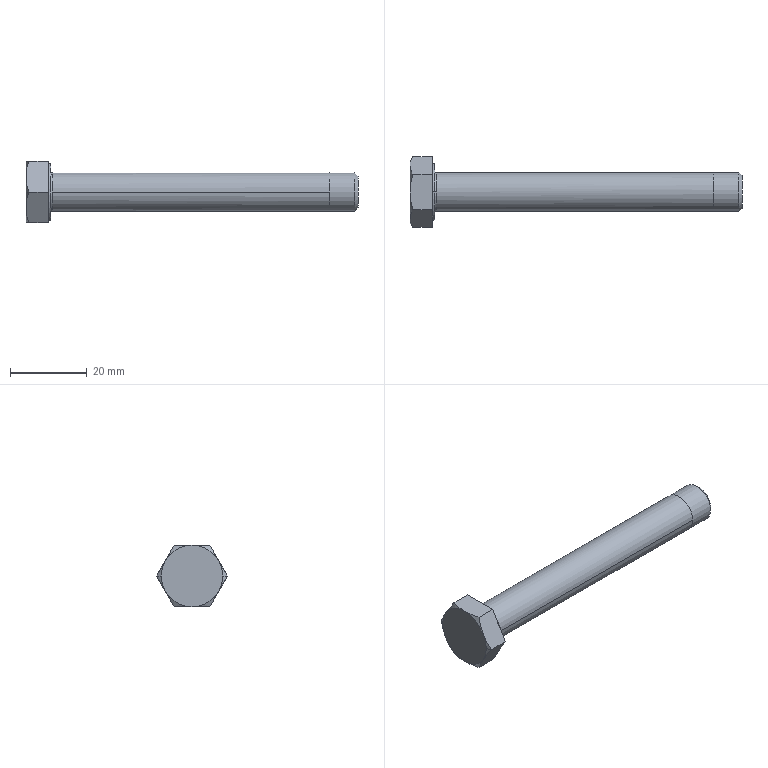Part | NX | features BREP 1, MOVE_FACE 1, REPLACE_FACE 1 | 1 solid | 27 faces | box 86.4 x 18.475 x 16 mm | volume 7660 mm3 | cone 10 | plane 10 | torus 4 | cylinder 3 | commonest cylinder face diameters 10 x3
STEP:
#1=CARTESIAN_POINT('',(-5.085,-9.238,0.));
#2=VERTEX_POINT('',#1);
#3=CARTESIAN_POINT('',(-5.8,-8.,0.));
#4=VERTEX_POINT('',#3);
#5=CARTESIAN_POINT('',(-5.442,-8.62,0.));
#6=DIRECTION('',(-0.5,0.866,0.));
#7=VECTOR('',#6,1000.);
#8=LINE('',#5,#7);
#9=EDGE_CURVE('',#2,#4,#8,.T.);
#10=ORIENTED_EDGE('',*,*,#9,.F.);
#11=CARTESIAN_POINT('',(-5.8,-6.928,4.));
#12=VERTEX_POINT('',#11);
#13=CARTESIAN_POINT('',(-5.084,-9.24,-0.004148));
#14=CARTESIAN_POINT('',(-5.8,-8.001,2.142));
#15=CARTESIAN_POINT('',(-5.8,-6.928,4.));
#16=CARTESIAN_POINT('',(-5.8,-5.855,5.858));
#17=CARTESIAN_POINT('',(-5.084,-4.616,8.004));
#18=(BOUNDED_CURVE()B_SPLINE_CURVE(2,(#13,#14,#15,#16,#17),.UNSPECIFIED.,.F.,.F.)B_SPLINE_CURVE_WITH_KNOTS((3,2,3),(0.,0.5,1.),.PIECEWISE_BEZIER_KNOTS.)CURVE()GEOMETRIC_REPRESENTATION_ITEM()RATIONAL_B_SPLINE_CURVE((1.,1.038,1.,1.038,1.))REPRESENTATION_ITEM(''));
#19=EDGE_CURVE('',#2,#12,#18,.T.);
#20=ORIENTED_EDGE('',*,*,#19,.T.);
#21=CARTESIAN_POINT('',(-5.8,0.,0.));
#22=DIRECTION('',(1.,0.,0.));
#23=DIRECTION('',(0.,1.,0.));
#24=AXIS2_PLACEMENT_3D('',#21,#22,#23);
#25=CIRCLE('',#24,8.);
#26=EDGE_CURVE('',#12,#4,#25,.T.);
#27=ORIENTED_EDGE('',*,*,#26,.T.);
#28=EDGE_LOOP('',(#10,#20,#27));
#29=FACE_BOUND('',#28,.T.);
#30=CARTESIAN_POINT('',(-5.442,0.,0.));
#31=DIRECTION('',(1.,0.,0.));
#32=DIRECTION('',(0.,-1.,0.));
#33=AXIS2_PLACEMENT_3D('',#30,#31,#32);
#34=CONICAL_SURFACE('',#33,8.62,1.047);
#35=ADVANCED_FACE('',(#29),#34,.T.);
#36=CARTESIAN_POINT('',(-5.8,8.,0.));
#37=VERTEX_POINT('',#36);
#38=CARTESIAN_POINT('',(-5.085,9.238,0.));
#39=VERTEX_POINT('',#38);
#40=CARTESIAN_POINT('',(-5.442,8.62,0.));
#41=DIRECTION('',(0.5,0.866,0.));
#42=VECTOR('',#41,1000.);
#43=LINE('',#40,#42);
#44=EDGE_CURVE('',#37,#39,#43,.T.);
#45=ORIENTED_EDGE('',*,*,#44,.F.);
#46=CARTESIAN_POINT('',(-5.8,6.928,4.));
#47=VERTEX_POINT('',#46);
#48=CARTESIAN_POINT('',(-5.8,0.,0.));
#49=DIRECTION('',(1.,0.,0.));
#50=DIRECTION('',(0.,1.,0.));
#51=AXIS2_PLACEMENT_3D('',#48,#49,#50);
#52=CIRCLE('',#51,8.);
#53=EDGE_CURVE('',#37,#47,#52,.T.);
#54=ORIENTED_EDGE('',*,*,#53,.T.);
#55=CARTESIAN_POINT('',(-5.084,4.616,8.004));
#56=CARTESIAN_POINT('',(-5.8,5.855,5.858));
#57=CARTESIAN_POINT('',(-5.8,6.928,4.));
#58=CARTESIAN_POINT('',(-5.8,8.001,2.142));
#59=CARTESIAN_POINT('',(-5.084,9.24,-0.004148));
#60=(BOUNDED_CURVE()B_SPLINE_CURVE(2,(#55,#56,#57,#58,#59),.UNSPECIFIED.,.F.,.F.)B_SPLINE_CURVE_WITH_KNOTS((3,2,3),(0.,0.5,1.),.PIECEWISE_BEZIER_KNOTS.)CURVE()GEOMETRIC_REPRESENTATION_ITEM()RATIONAL_B_SPLINE_CURVE((1.,1.038,1.,1.038,1.))REPRESENTATION_ITEM(''));
#61=EDGE_CURVE('',#47,#39,#60,.T.);
#62=ORIENTED_EDGE('',*,*,#61,.T.);
#63=EDGE_LOOP('',(#45,#54,#62));
#64=FACE_BOUND('',#63,.T.);
#65=CARTESIAN_POINT('',(-5.442,0.,0.));
#66=DIRECTION('',(1.,0.,0.));
#67=DIRECTION('',(0.,-1.,0.));
#68=AXIS2_PLACEMENT_3D('',#65,#66,#67);
#69=CONICAL_SURFACE('',#68,8.62,1.047);
#70=ADVANCED_FACE('',(#64),#69,.T.);
#71=CARTESIAN_POINT('',(79.788,5.,0.));
#72=VERTEX_POINT('',#71);
#73=CARTESIAN_POINT('',(80.6,4.188,0.));
#74=VERTEX_POINT('',#73);
#75=CARTESIAN_POINT('',(80.194,4.594,0.));
#76=DIRECTION('',(0.7071,-0.7071,0.));
#77=VECTOR('',#76,1000.);
#78=LINE('',#75,#77);
#79=EDGE_CURVE('',#72,#74,#78,.T.);
#80=ORIENTED_EDGE('',*,*,#79,.F.);
#81=CARTESIAN_POINT('',(79.788,-5.,0.));
#82=VERTEX_POINT('',#81);
#83=CARTESIAN_POINT('',(79.788,0.,0.));
#84=DIRECTION('',(1.,0.,0.));
#85=DIRECTION('',(0.,1.,0.));
#86=AXIS2_PLACEMENT_3D('',#83,#84,#85);
#87=CIRCLE('',#86,5.);
#88=EDGE_CURVE('',#72,#82,#87,.T.);
#89=ORIENTED_EDGE('',*,*,#88,.T.);
#90=CARTESIAN_POINT('',(80.6,-4.188,0.));
#91=VERTEX_POINT('',#90);
#92=CARTESIAN_POINT('',(80.194,-4.594,0.));
#93=DIRECTION('',(-0.7071,-0.7071,0.));
#94=VECTOR('',#93,1000.);
#95=LINE('',#92,#94);
#96=EDGE_CURVE('',#91,#82,#95,.T.);
#97=ORIENTED_EDGE('',*,*,#96,.F.);
#98=CARTESIAN_POINT('',(80.6,0.,0.));
#99=DIRECTION('',(1.,0.,0.));
#100=DIRECTION('',(0.,1.,0.));
#101=AXIS2_PLACEMENT_3D('',#98,#99,#100);
#102=CIRCLE('',#101,4.188);
#103=EDGE_CURVE('',#74,#91,#102,.T.);
#104=ORIENTED_EDGE('',*,*,#103,.F.);
#105=EDGE_LOOP('',(#80,#89,#97,#104));
#106=FACE_BOUND('',#105,.T.);
#107=CARTESIAN_POINT('',(80.194,0.,0.));
#108=DIRECTION('',(-1.,0.,0.));
#109=DIRECTION('',(0.,-1.,0.));
#110=AXIS2_PLACEMENT_3D('',#107,#108,#109);
#111=CONICAL_SURFACE('',#110,4.594,0.7854);
#112=ADVANCED_FACE('',(#106),#111,.T.);
#113=ORIENTED_EDGE('',*,*,#88,.F.);
#114=CARTESIAN_POINT('',(79.788,0.,0.));
#115=DIRECTION('',(1.,0.,0.));
#116=DIRECTION('',(0.,1.,0.));
#117=AXIS2_PLACEMENT_3D('',#114,#115,#116);
#118=CIRCLE('',#117,5.);
#119=EDGE_CURVE('',#82,#72,#118,.T.);
#120=ORIENTED_EDGE('',*,*,#119,.F.);
#121=EDGE_LOOP('',(#113,#120));
#122=FACE_BOUND('',#121,.T.);
#123=CARTESIAN_POINT('',(73.194,5.,0.));
#124=VERTEX_POINT('',#123);
#125=CARTESIAN_POINT('',(73.194,-5.,0.));
#126=VERTEX_POINT('',#125);
#127=CARTESIAN_POINT('',(73.194,0.,0.));
#128=DIRECTION('',(1.,0.,0.));
#129=DIRECTION('',(0.,1.,0.));
#130=AXIS2_PLACEMENT_3D('',#127,#128,#129);
#131=CIRCLE('',#130,5.);
#132=EDGE_CURVE('',#124,#126,#131,.T.);
#133=ORIENTED_EDGE('',*,*,#132,.T.);
#134=CARTESIAN_POINT('',(73.194,0.,0.));
#135=DIRECTION('',(1.,0.,0.));
#136=DIRECTION('',(0.,1.,0.));
#137=AXIS2_PLACEMENT_3D('',#134,#135,#136);
#138=CIRCLE('',#137,5.);
#139=EDGE_CURVE('',#126,#124,#138,.T.);
#140=ORIENTED_EDGE('',*,*,#139,.T.);
#141=EDGE_LOOP('',(#133,#140));
#142=FACE_BOUND('',#141,.T.);
#143=CARTESIAN_POINT('',(87.194,0.,0.));
#144=DIRECTION('',(1.,0.,0.));
#145=DIRECTION('',(0.,-1.,0.));
#146=AXIS2_PLACEMENT_3D('',#143,#144,#145);
#147=CYLINDRICAL_SURFACE('',#146,5.);
#148=ADVANCED_FACE('',(#122,#142),#147,.T.);
#149=CARTESIAN_POINT('',(1.,5.,0.));
#150=VERTEX_POINT('',#149);
#151=CARTESIAN_POINT('',(37.097,5.,0.));
#152=DIRECTION('',(1.,0.,0.));
#153=VECTOR('',#152,1000.);
#154=LINE('',#151,#153);
#155=EDGE_CURVE('',#150,#124,#154,.T.);
#156=ORIENTED_EDGE('',*,*,#155,.F.);
#157=CARTESIAN_POINT('',(1.,0.,5.));
#158=VERTEX_POINT('',#157);
#159=CARTESIAN_POINT('',(1.,0.,0.));
#160=DIRECTION('',(1.,0.,0.));
#161=DIRECTION('',(0.,1.,0.));
#162=AXIS2_PLACEMENT_3D('',#159,#160,#161);
#163=CIRCLE('',#162,5.);
#164=EDGE_CURVE('',#150,#158,#163,.T.);
#165=ORIENTED_EDGE('',*,*,#164,.T.);
#166=CARTESIAN_POINT('',(1.,-5.,0.));
#167=VERTEX_POINT('',#166);
#168=CARTESIAN_POINT('',(1.,0.,0.));
#169=DIRECTION('',(1.,0.,0.));
#170=DIRECTION('',(0.,1.,0.));
#171=AXIS2_PLACEMENT_3D('',#168,#169,#170);
#172=CIRCLE('',#171,5.);
#173=EDGE_CURVE('',#158,#167,#172,.T.);
#174=ORIENTED_EDGE('',*,*,#173,.T.);
#175=CARTESIAN_POINT('',(37.097,-5.,0.));
#176=DIRECTION('',(-1.,0.,0.));
#177=VECTOR('',#176,1000.);
#178=LINE('',#175,#177);
#179=EDGE_CURVE('',#126,#167,#178,.T.);
#180=ORIENTED_EDGE('',*,*,#179,.F.);
#181=ORIENTED_EDGE('',*,*,#132,.F.);
#182=EDGE_LOOP('',(#156,#165,#174,#180,#181));
#183=FACE_BOUND('',#182,.T.);
#184=CARTESIAN_POINT('',(37.097,0.,0.));
#185=DIRECTION('',(1.,0.,0.));
#186=DIRECTION('',(0.,-1.,0.));
#187=AXIS2_PLACEMENT_3D('',#184,#185,#186);
#188=CYLINDRICAL_SURFACE('',#187,5.);
#189=ADVANCED_FACE('',(#183),#188,.T.);
#190=CARTESIAN_POINT('',(0.6,0.,5.4));
#191=VERTEX_POINT('',#190);
#192=CARTESIAN_POINT('',(1.,0.,5.4));
#193=DIRECTION('',(0.,-1.,0.));
#194=DIRECTION('',(0.,0.,1.));
#195=AXIS2_PLACEMENT_3D('',#192,#193,#194);
#196=CIRCLE('',#195,0.4);
#197=EDGE_CURVE('',#191,#158,#196,.T.);
#198=ORIENTED_EDGE('',*,*,#197,.F.);
#199=CARTESIAN_POINT('',(0.6,0.,-5.4));
#200=VERTEX_POINT('',#199);
#201=CARTESIAN_POINT('',(0.6,0.,0.));
#202=DIRECTION('',(1.,0.,0.));
#203=DIRECTION('',(0.,1.,0.));
#204=AXIS2_PLACEMENT_3D('',#201,#202,#203);
#205=CIRCLE('',#204,5.4);
#206=EDGE_CURVE('',#191,#200,#205,.T.);
#207=ORIENTED_EDGE('',*,*,#206,.T.);
#208=CARTESIAN_POINT('',(1.,0.,-5.));
#209=VERTEX_POINT('',#208);
#210=CARTESIAN_POINT('',(1.,0.,-5.4));
#211=DIRECTION('',(0.,-1.,0.));
#212=DIRECTION('',(0.,0.,-1.));
#213=AXIS2_PLACEMENT_3D('',#210,#211,#212);
#214=CIRCLE('',#213,0.4);
#215=EDGE_CURVE('',#209,#200,#214,.T.);
#216=ORIENTED_EDGE('',*,*,#215,.F.);
#217=CARTESIAN_POINT('',(1.,0.,0.));
#218=DIRECTION('',(1.,0.,0.));
#219=DIRECTION('',(0.,1.,0.));
#220=AXIS2_PLACEMENT_3D('',#217,#218,#219);
#221=CIRCLE('',#220,5.);
#222=EDGE_CURVE('',#167,#209,#221,.T.);
#223=ORIENTED_EDGE('',*,*,#222,.F.);
#224=ORIENTED_EDGE('',*,*,#173,.F.);
#225=EDGE_LOOP('',(#198,#207,#216,#223,#224));
#226=FACE_BOUND('',#225,.T.);
#227=CARTESIAN_POINT('',(1.,0.,0.));
#228=DIRECTION('',(1.,0.,0.));
#229=DIRECTION('',(0.,0.,1.));
#230=AXIS2_PLACEMENT_3D('',#227,#228,#229);
#231=TOROIDAL_SURFACE('',#230,5.4,0.4);
#232=ADVANCED_FACE('',(#226),#231,.F.);
#233=CARTESIAN_POINT('',(0.,0.,7.915));
#234=VERTEX_POINT('',#233);
#235=CARTESIAN_POINT('',(0.6,0.,7.315));
#236=VERTEX_POINT('',#235);
#237=CARTESIAN_POINT('',(0.6,0.,7.915));
#238=DIRECTION('',(0.,-1.,0.));
#239=DIRECTION('',(0.,0.,1.));
#240=AXIS2_PLACEMENT_3D('',#237,#238,#239);
#241=CIRCLE('',#240,0.6);
#242=EDGE_CURVE('',#234,#236,#241,.T.);
#243=ORIENTED_EDGE('',*,*,#242,.F.);
#244=CARTESIAN_POINT('',(0.,0.,-7.915));
#245=VERTEX_POINT('',#244);
#246=CARTESIAN_POINT('',(0.,0.,0.));
#247=DIRECTION('',(-1.,0.,0.));
#248=DIRECTION('',(0.,1.,0.));
#249=AXIS2_PLACEMENT_3D('',#246,#247,#248);
#250=CIRCLE('',#249,7.915);
#251=EDGE_CURVE('',#245,#234,#250,.T.);
#252=ORIENTED_EDGE('',*,*,#251,.F.);
#253=CARTESIAN_POINT('',(0.6,0.,-7.315));
#254=VERTEX_POINT('',#253);
#255=CARTESIAN_POINT('',(0.6,0.,-7.915));
#256=DIRECTION('',(0.,-1.,0.));
#257=DIRECTION('',(0.,0.,-1.));
#258=AXIS2_PLACEMENT_3D('',#255,#256,#257);
#259=CIRCLE('',#258,0.6);
#260=EDGE_CURVE('',#254,#245,#259,.T.);
#261=ORIENTED_EDGE('',*,*,#260,.F.);
#262=CARTESIAN_POINT('',(0.6,0.,0.));
#263=DIRECTION('',(1.,0.,0.));
#264=DIRECTION('',(0.,1.,0.));
#265=AXIS2_PLACEMENT_3D('',#262,#263,#264);
#266=CIRCLE('',#265,7.315);
#267=EDGE_CURVE('',#236,#254,#266,.T.);
#268=ORIENTED_EDGE('',*,*,#267,.F.);
#269=EDGE_LOOP('',(#243,#252,#261,#268));
#270=FACE_BOUND('',#269,.T.);
#271=CARTESIAN_POINT('',(0.6,0.,0.));
#272=DIRECTION('',(1.,0.,0.));
#273=DIRECTION('',(0.,0.,1.));
#274=AXIS2_PLACEMENT_3D('',#271,#272,#273);
#275=TOROIDAL_SURFACE('',#274,7.915,0.6);
#276=ADVANCED_FACE('',(#270),#275,.F.);
#277=ORIENTED_EDGE('',*,*,#242,.T.);
#278=CARTESIAN_POINT('',(0.6,7.315,0.));
#279=VERTEX_POINT('',#278);
#280=CARTESIAN_POINT('',(0.6,0.,0.));
#281=DIRECTION('',(1.,0.,0.));
#282=DIRECTION('',(0.,1.,0.));
#283=AXIS2_PLACEMENT_3D('',#280,#281,#282);
#284=CIRCLE('',#283,7.315);
#285=EDGE_CURVE('',#279,#236,#284,.T.);
#286=ORIENTED_EDGE('',*,*,#285,.F.);
#287=CARTESIAN_POINT('',(0.6,0.,0.));
#288=DIRECTION('',(1.,0.,0.));
#289=DIRECTION('',(0.,1.,0.));
#290=AXIS2_PLACEMENT_3D('',#287,#288,#289);
#291=CIRCLE('',#290,7.315);
#292=EDGE_CURVE('',#254,#279,#291,.T.);
#293=ORIENTED_EDGE('',*,*,#292,.F.);
#294=ORIENTED_EDGE('',*,*,#260,.T.);
#295=CARTESIAN_POINT('',(0.,7.915,0.));
#296=VERTEX_POINT('',#295);
#297=CARTESIAN_POINT('',(0.,0.,0.));
#298=DIRECTION('',(-1.,0.,0.));
#299=DIRECTION('',(0.,1.,0.));
#300=AXIS2_PLACEMENT_3D('',#297,#298,#299);
#301=CIRCLE('',#300,7.915);
#302=EDGE_CURVE('',#296,#245,#301,.T.);
#303=ORIENTED_EDGE('',*,*,#302,.F.);
#304=CARTESIAN_POINT('',(0.,0.,0.));
#305=DIRECTION('',(-1.,0.,0.));
#306=DIRECTION('',(0.,1.,0.));
#307=AXIS2_PLACEMENT_3D('',#304,#305,#306);
#308=CIRCLE('',#307,7.915);
#309=EDGE_CURVE('',#234,#296,#308,.T.);
#310=ORIENTED_EDGE('',*,*,#309,.F.);
#311=EDGE_LOOP('',(#277,#286,#293,#294,#303,#310));
#312=FACE_BOUND('',#311,.T.);
#313=CARTESIAN_POINT('',(0.6,0.,0.));
#314=DIRECTION('',(1.,0.,0.));
#315=DIRECTION('',(0.,0.,1.));
#316=AXIS2_PLACEMENT_3D('',#313,#314,#315);
#317=TOROIDAL_SURFACE('',#316,7.915,0.6);
#318=ADVANCED_FACE('',(#312),#317,.F.);
#319=CARTESIAN_POINT('',(0.6,5.4,0.));
#320=VERTEX_POINT('',#319);
#321=CARTESIAN_POINT('',(0.6,0.,0.));
#322=DIRECTION('',(1.,0.,0.));
#323=DIRECTION('',(0.,1.,0.));
#324=AXIS2_PLACEMENT_3D('',#321,#322,#323);
#325=CIRCLE('',#324,5.4);
#326=EDGE_CURVE('',#320,#191,#325,.T.);
#327=ORIENTED_EDGE('',*,*,#326,.F.);
#328=CARTESIAN_POINT('',(0.6,0.,0.));
#329=DIRECTION('',(1.,0.,0.));
#330=DIRECTION('',(0.,1.,0.));
#331=AXIS2_PLACEMENT_3D('',#328,#329,#330);
#332=CIRCLE('',#331,5.4);
#333=EDGE_CURVE('',#200,#320,#332,.T.);
#334=ORIENTED_EDGE('',*,*,#333,.F.);
#335=ORIENTED_EDGE('',*,*,#206,.F.);
#336=EDGE_LOOP('',(#327,#334,#335));
#337=FACE_BOUND('',#336,.T.);
#338=ORIENTED_EDGE('',*,*,#285,.T.);
#339=ORIENTED_EDGE('',*,*,#267,.T.);
#340=ORIENTED_EDGE('',*,*,#292,.T.);
#341=EDGE_LOOP('',(#338,#339,#340));
#342=FACE_BOUND('',#341,.T.);
#343=CARTESIAN_POINT('',(0.6,6.357,0.));
#344=DIRECTION('',(1.,0.,0.));
#345=DIRECTION('',(0.,-1.,0.));
#346=AXIS2_PLACEMENT_3D('',#343,#344,#345);
#347=PLANE('',#346);
#348=ADVANCED_FACE('',(#337,#342),#347,.T.);
#349=ORIENTED_EDGE('',*,*,#197,.T.);
#350=ORIENTED_EDGE('',*,*,#164,.F.);
#351=CARTESIAN_POINT('',(1.,0.,0.));
#352=DIRECTION('',(1.,0.,0.));
#353=DIRECTION('',(0.,1.,0.));
#354=AXIS2_PLACEMENT_3D('',#351,#352,#353);
#355=CIRCLE('',#354,5.);
#356=EDGE_CURVE('',#209,#150,#355,.T.);
#357=ORIENTED_EDGE('',*,*,#356,.F.);
#358=ORIENTED_EDGE('',*,*,#215,.T.);
#359=ORIENTED_EDGE('',*,*,#333,.T.);
#360=ORIENTED_EDGE('',*,*,#326,.T.);
#361=EDGE_LOOP('',(#349,#350,#357,#358,#359,#360));
#362=FACE_BOUND('',#361,.T.);
#363=CARTESIAN_POINT('',(1.,0.,0.));
#364=DIRECTION('',(1.,0.,0.));
#365=DIRECTION('',(0.,0.,1.));
#366=AXIS2_PLACEMENT_3D('',#363,#364,#365);
#367=TOROIDAL_SURFACE('',#366,5.4,0.4);
#368=ADVANCED_FACE('',(#362),#367,.F.);
#369=ORIENTED_EDGE('',*,*,#155,.T.);
#370=ORIENTED_EDGE('',*,*,#139,.F.);
#371=ORIENTED_EDGE('',*,*,#179,.T.);
#372=ORIENTED_EDGE('',*,*,#222,.T.);
#373=ORIENTED_EDGE('',*,*,#356,.T.);
#374=EDGE_LOOP('',(#369,#370,#371,#372,#373));
#375=FACE_BOUND('',#374,.T.);
#376=CARTESIAN_POINT('',(37.097,0.,0.));
#377=DIRECTION('',(1.,0.,0.));
#378=DIRECTION('',(0.,-1.,0.));
#379=AXIS2_PLACEMENT_3D('',#376,#377,#378);
#380=CYLINDRICAL_SURFACE('',#379,5.);
#381=ADVANCED_FACE('',(#375),#380,.T.);
#382=ORIENTED_EDGE('',*,*,#79,.T.);
#383=CARTESIAN_POINT('',(80.6,0.,0.));
#384=DIRECTION('',(1.,0.,0.));
#385=DIRECTION('',(0.,1.,0.));
#386=AXIS2_PLACEMENT_3D('',#383,#384,#385);
#387=CIRCLE('',#386,4.188);
#388=EDGE_CURVE('',#91,#74,#387,.T.);
#389=ORIENTED_EDGE('',*,*,#388,.F.);
#390=ORIENTED_EDGE('',*,*,#96,.T.);
#391=ORIENTED_EDGE('',*,*,#119,.T.);
#392=EDGE_LOOP('',(#382,#389,#390,#391));
#393=FACE_BOUND('',#392,.T.);
#394=CARTESIAN_POINT('',(80.194,0.,0.));
#395=DIRECTION('',(-1.,0.,0.));
#396=DIRECTION('',(0.,-1.,0.));
#397=AXIS2_PLACEMENT_3D('',#394,#395,#396);
#398=CONICAL_SURFACE('',#397,4.594,0.7854);
#399=ADVANCED_FACE('',(#393),#398,.T.);
#400=ORIENTED_EDGE('',*,*,#103,.T.);
#401=ORIENTED_EDGE('',*,*,#388,.T.);
#402=EDGE_LOOP('',(#400,#401));
#403=FACE_BOUND('',#402,.T.);
#404=CARTESIAN_POINT('',(80.6,2.094,0.));
#405=DIRECTION('',(1.,0.,0.));
#406=DIRECTION('',(0.,-1.,0.));
#407=AXIS2_PLACEMENT_3D('',#404,#405,#406);
#408=PLANE('',#407);
#409=ADVANCED_FACE('',(#403),#408,.T.);
#410=CARTESIAN_POINT('',(-5.085,-4.619,8.));
#411=VERTEX_POINT('',#410);
#412=CARTESIAN_POINT('',(-5.8,0.,8.));
#413=VERTEX_POINT('',#412);
#414=CARTESIAN_POINT('',(-5.084,-4.624,8.));
#415=CARTESIAN_POINT('',(-5.8,-2.146,8.));
#416=CARTESIAN_POINT('',(-5.8,0.,8.));
#417=CARTESIAN_POINT('',(-5.8,2.146,8.));
#418=CARTESIAN_POINT('',(-5.084,4.624,8.));
#419=(BOUNDED_CURVE()B_SPLINE_CURVE(2,(#414,#415,#416,#417,#418),.UNSPECIFIED.,.F.,.F.)B_SPLINE_CURVE_WITH_KNOTS((3,2,3),(0.,0.5,1.),.PIECEWISE_BEZIER_KNOTS.)CURVE()GEOMETRIC_REPRESENTATION_ITEM()RATIONAL_B_SPLINE_CURVE((1.,1.038,1.,1.038,1.))REPRESENTATION_ITEM(''));
#420=EDGE_CURVE('',#411,#413,#419,.T.);
#421=ORIENTED_EDGE('',*,*,#420,.T.);
#422=CARTESIAN_POINT('',(-5.8,0.,0.));
#423=DIRECTION('',(1.,0.,0.));
#424=DIRECTION('',(0.,1.,0.));
#425=AXIS2_PLACEMENT_3D('',#422,#423,#424);
#426=CIRCLE('',#425,8.);
#427=EDGE_CURVE('',#413,#12,#426,.T.);
#428=ORIENTED_EDGE('',*,*,#427,.T.);
#429=CARTESIAN_POINT('',(-5.084,-9.24,-0.004148));
#430=CARTESIAN_POINT('',(-5.8,-8.001,2.142));
#431=CARTESIAN_POINT('',(-5.8,-6.928,4.));
#432=CARTESIAN_POINT('',(-5.8,-5.855,5.858));
#433=CARTESIAN_POINT('',(-5.084,-4.616,8.004));
#434=(BOUNDED_CURVE()B_SPLINE_CURVE(2,(#429,#430,#431,#432,#433),.UNSPECIFIED.,.F.,.F.)B_SPLINE_CURVE_WITH_KNOTS((3,2,3),(0.,0.5,1.),.PIECEWISE_BEZIER_KNOTS.)CURVE()GEOMETRIC_REPRESENTATION_ITEM()RATIONAL_B_SPLINE_CURVE((1.,1.038,1.,1.038,1.))REPRESENTATION_ITEM(''));
#435=EDGE_CURVE('',#12,#411,#434,.T.);
#436=ORIENTED_EDGE('',*,*,#435,.T.);
#437=EDGE_LOOP('',(#421,#428,#436));
#438=FACE_BOUND('',#437,.T.);
#439=CARTESIAN_POINT('',(-5.442,0.,0.));
#440=DIRECTION('',(1.,0.,0.));
#441=DIRECTION('',(0.,-1.,0.));
#442=AXIS2_PLACEMENT_3D('',#439,#440,#441);
#443=CONICAL_SURFACE('',#442,8.62,1.047);
#444=ADVANCED_FACE('',(#438),#443,.T.);
#445=CARTESIAN_POINT('',(-5.085,4.619,8.));
#446=VERTEX_POINT('',#445);
#447=CARTESIAN_POINT('',(-5.084,4.616,8.004));
#448=CARTESIAN_POINT('',(-5.8,5.855,5.858));
#449=CARTESIAN_POINT('',(-5.8,6.928,4.));
#450=CARTESIAN_POINT('',(-5.8,8.001,2.142));
#451=CARTESIAN_POINT('',(-5.084,9.24,-0.004148));
#452=(BOUNDED_CURVE()B_SPLINE_CURVE(2,(#447,#448,#449,#450,#451),.UNSPECIFIED.,.F.,.F.)B_SPLINE_CURVE_WITH_KNOTS((3,2,3),(0.,0.5,1.),.PIECEWISE_BEZIER_KNOTS.)CURVE()GEOMETRIC_REPRESENTATION_ITEM()RATIONAL_B_SPLINE_CURVE((1.,1.038,1.,1.038,1.))REPRESENTATION_ITEM(''));
#453=EDGE_CURVE('',#446,#47,#452,.T.);
#454=ORIENTED_EDGE('',*,*,#453,.T.);
#455=CARTESIAN_POINT('',(-5.8,0.,0.));
#456=DIRECTION('',(1.,0.,0.));
#457=DIRECTION('',(0.,1.,0.));
#458=AXIS2_PLACEMENT_3D('',#455,#456,#457);
#459=CIRCLE('',#458,8.);
#460=EDGE_CURVE('',#47,#413,#459,.T.);
#461=ORIENTED_EDGE('',*,*,#460,.T.);
#462=CARTESIAN_POINT('',(-5.084,-4.624,8.));
#463=CARTESIAN_POINT('',(-5.8,-2.146,8.));
#464=CARTESIAN_POINT('',(-5.8,0.,8.));
#465=CARTESIAN_POINT('',(-5.8,2.146,8.));
#466=CARTESIAN_POINT('',(-5.084,4.624,8.));
#467=(BOUNDED_CURVE()B_SPLINE_CURVE(2,(#462,#463,#464,#465,#466),.UNSPECIFIED.,.F.,.F.)B_SPLINE_CURVE_WITH_KNOTS((3,2,3),(0.,0.5,1.),.PIECEWISE_BEZIER_KNOTS.)CURVE()GEOMETRIC_REPRESENTATION_ITEM()RATIONAL_B_SPLINE_CURVE((1.,1.038,1.,1.038,1.))REPRESENTATION_ITEM(''));
#468=EDGE_CURVE('',#413,#446,#467,.T.);
#469=ORIENTED_EDGE('',*,*,#468,.T.);
#470=EDGE_LOOP('',(#454,#461,#469));
#471=FACE_BOUND('',#470,.T.);
#472=CARTESIAN_POINT('',(-5.442,0.,0.));
#473=DIRECTION('',(1.,0.,0.));
#474=DIRECTION('',(0.,-1.,0.));
#475=AXIS2_PLACEMENT_3D('',#472,#473,#474);
#476=CONICAL_SURFACE('',#475,8.62,1.047);
#477=ADVANCED_FACE('',(#471),#476,.T.);
#478=ORIENTED_EDGE('',*,*,#44,.T.);
#479=CARTESIAN_POINT('',(-5.8,6.928,-4.));
#480=VERTEX_POINT('',#479);
#481=CARTESIAN_POINT('',(-5.084,9.24,0.004148));
#482=CARTESIAN_POINT('',(-5.8,8.001,-2.142));
#483=CARTESIAN_POINT('',(-5.8,6.928,-4.));
#484=CARTESIAN_POINT('',(-5.8,5.855,-5.858));
#485=CARTESIAN_POINT('',(-5.084,4.616,-8.004));
#486=(BOUNDED_CURVE()B_SPLINE_CURVE(2,(#481,#482,#483,#484,#485),.UNSPECIFIED.,.F.,.F.)B_SPLINE_CURVE_WITH_KNOTS((3,2,3),(0.,0.5,1.),.PIECEWISE_BEZIER_KNOTS.)CURVE()GEOMETRIC_REPRESENTATION_ITEM()RATIONAL_B_SPLINE_CURVE((1.,1.038,1.,1.038,1.))REPRESENTATION_ITEM(''));
#487=EDGE_CURVE('',#39,#480,#486,.T.);
#488=ORIENTED_EDGE('',*,*,#487,.T.);
#489=CARTESIAN_POINT('',(-5.8,0.,0.));
#490=DIRECTION('',(1.,0.,0.));
#491=DIRECTION('',(0.,1.,0.));
#492=AXIS2_PLACEMENT_3D('',#489,#490,#491);
#493=CIRCLE('',#492,8.);
#494=EDGE_CURVE('',#480,#37,#493,.T.);
#495=ORIENTED_EDGE('',*,*,#494,.T.);
#496=EDGE_LOOP('',(#478,#488,#495));
#497=FACE_BOUND('',#496,.T.);
#498=CARTESIAN_POINT('',(-5.442,0.,0.));
#499=DIRECTION('',(1.,0.,0.));
#500=DIRECTION('',(0.,-1.,0.));
#501=AXIS2_PLACEMENT_3D('',#498,#499,#500);
#502=CONICAL_SURFACE('',#501,8.62,1.047);
#503=ADVANCED_FACE('',(#497),#502,.T.);
#504=CARTESIAN_POINT('',(-5.085,4.619,-8.));
#505=VERTEX_POINT('',#504);
#506=CARTESIAN_POINT('',(-5.084,9.24,0.004148));
#507=CARTESIAN_POINT('',(-5.8,8.001,-2.142));
#508=CARTESIAN_POINT('',(-5.8,6.928,-4.));
#509=CARTESIAN_POINT('',(-5.8,5.855,-5.858));
#510=CARTESIAN_POINT('',(-5.084,4.616,-8.004));
#511=(BOUNDED_CURVE()B_SPLINE_CURVE(2,(#506,#507,#508,#509,#510),.UNSPECIFIED.,.F.,.F.)B_SPLINE_CURVE_WITH_KNOTS((3,2,3),(0.,0.5,1.),.PIECEWISE_BEZIER_KNOTS.)CURVE()GEOMETRIC_REPRESENTATION_ITEM()RATIONAL_B_SPLINE_CURVE((1.,1.038,1.,1.038,1.))REPRESENTATION_ITEM(''));
#512=EDGE_CURVE('',#480,#505,#511,.T.);
#513=ORIENTED_EDGE('',*,*,#512,.T.);
#514=CARTESIAN_POINT('',(-5.8,0.,-8.));
#515=VERTEX_POINT('',#514);
#516=CARTESIAN_POINT('',(-5.084,4.624,-8.));
#517=CARTESIAN_POINT('',(-5.8,2.146,-8.));
#518=CARTESIAN_POINT('',(-5.8,0.,-8.));
#519=CARTESIAN_POINT('',(-5.8,-2.146,-8.));
#520=CARTESIAN_POINT('',(-5.084,-4.624,-8.));
#521=(BOUNDED_CURVE()B_SPLINE_CURVE(2,(#516,#517,#518,#519,#520),.UNSPECIFIED.,.F.,.F.)B_SPLINE_CURVE_WITH_KNOTS((3,2,3),(0.,0.5,1.),.PIECEWISE_BEZIER_KNOTS.)CURVE()GEOMETRIC_REPRESENTATION_ITEM()RATIONAL_B_SPLINE_CURVE((1.,1.038,1.,1.038,1.))REPRESENTATION_ITEM(''));
#522=EDGE_CURVE('',#505,#515,#521,.T.);
#523=ORIENTED_EDGE('',*,*,#522,.T.);
#524=CARTESIAN_POINT('',(-5.8,0.,0.));
#525=DIRECTION('',(1.,0.,0.));
#526=DIRECTION('',(0.,1.,0.));
#527=AXIS2_PLACEMENT_3D('',#524,#525,#526);
#528=CIRCLE('',#527,8.);
#529=EDGE_CURVE('',#515,#480,#528,.T.);
#530=ORIENTED_EDGE('',*,*,#529,.T.);
#531=EDGE_LOOP('',(#513,#523,#530));
#532=FACE_BOUND('',#531,.T.);
#533=CARTESIAN_POINT('',(-5.442,0.,0.));
#534=DIRECTION('',(1.,0.,0.));
#535=DIRECTION('',(0.,-1.,0.));
#536=AXIS2_PLACEMENT_3D('',#533,#534,#535);
#537=CONICAL_SURFACE('',#536,8.62,1.047);
#538=ADVANCED_FACE('',(#532),#537,.T.);
#539=CARTESIAN_POINT('',(-5.085,-4.619,-8.));
#540=VERTEX_POINT('',#539);
#541=CARTESIAN_POINT('',(-5.084,4.624,-8.));
#542=CARTESIAN_POINT('',(-5.8,2.146,-8.));
#543=CARTESIAN_POINT('',(-5.8,0.,-8.));
#544=CARTESIAN_POINT('',(-5.8,-2.146,-8.));
#545=CARTESIAN_POINT('',(-5.084,-4.624,-8.));
#546=(BOUNDED_CURVE()B_SPLINE_CURVE(2,(#541,#542,#543,#544,#545),.UNSPECIFIED.,.F.,.F.)B_SPLINE_CURVE_WITH_KNOTS((3,2,3),(0.,0.5,1.),.PIECEWISE_BEZIER_KNOTS.)CURVE()GEOMETRIC_REPRESENTATION_ITEM()RATIONAL_B_SPLINE_CURVE((1.,1.038,1.,1.038,1.))REPRESENTATION_ITEM(''));
#547=EDGE_CURVE('',#515,#540,#546,.T.);
#548=ORIENTED_EDGE('',*,*,#547,.T.);
#549=CARTESIAN_POINT('',(-5.8,-6.928,-4.));
#550=VERTEX_POINT('',#549);
#551=CARTESIAN_POINT('',(-5.084,-4.616,-8.004));
#552=CARTESIAN_POINT('',(-5.8,-5.855,-5.858));
#553=CARTESIAN_POINT('',(-5.8,-6.928,-4.));
#554=CARTESIAN_POINT('',(-5.8,-8.001,-2.142));
#555=CARTESIAN_POINT('',(-5.084,-9.24,0.004148));
#556=(BOUNDED_CURVE()B_SPLINE_CURVE(2,(#551,#552,#553,#554,#555),.UNSPECIFIED.,.F.,.F.)B_SPLINE_CURVE_WITH_KNOTS((3,2,3),(0.,0.5,1.),.PIECEWISE_BEZIER_KNOTS.)CURVE()GEOMETRIC_REPRESENTATION_ITEM()RATIONAL_B_SPLINE_CURVE((1.,1.038,1.,1.038,1.))REPRESENTATION_ITEM(''));
#557=EDGE_CURVE('',#540,#550,#556,.T.);
#558=ORIENTED_EDGE('',*,*,#557,.T.);
#559=CARTESIAN_POINT('',(-5.8,0.,0.));
#560=DIRECTION('',(1.,0.,0.));
#561=DIRECTION('',(0.,1.,0.));
#562=AXIS2_PLACEMENT_3D('',#559,#560,#561);
#563=CIRCLE('',#562,8.);
#564=EDGE_CURVE('',#550,#515,#563,.T.);
#565=ORIENTED_EDGE('',*,*,#564,.T.);
#566=EDGE_LOOP('',(#548,#558,#565));
#567=FACE_BOUND('',#566,.T.);
#568=CARTESIAN_POINT('',(-5.442,0.,0.));
#569=DIRECTION('',(1.,0.,0.));
#570=DIRECTION('',(0.,-1.,0.));
#571=AXIS2_PLACEMENT_3D('',#568,#569,#570);
#572=CONICAL_SURFACE('',#571,8.62,1.047);
#573=ADVANCED_FACE('',(#567),#572,.T.);
#574=ORIENTED_EDGE('',*,*,#9,.T.);
#575=CARTESIAN_POINT('',(-5.8,0.,0.));
#576=DIRECTION('',(1.,0.,0.));
#577=DIRECTION('',(0.,1.,0.));
#578=AXIS2_PLACEMENT_3D('',#575,#576,#577);
#579=CIRCLE('',#578,8.);
#580=EDGE_CURVE('',#4,#550,#579,.T.);
#581=ORIENTED_EDGE('',*,*,#580,.T.);
#582=CARTESIAN_POINT('',(-5.084,-4.616,-8.004));
#583=CARTESIAN_POINT('',(-5.8,-5.855,-5.858));
#584=CARTESIAN_POINT('',(-5.8,-6.928,-4.));
#585=CARTESIAN_POINT('',(-5.8,-8.001,-2.142));
#586=CARTESIAN_POINT('',(-5.084,-9.24,0.004148));
#587=(BOUNDED_CURVE()B_SPLINE_CURVE(2,(#582,#583,#584,#585,#586),.UNSPECIFIED.,.F.,.F.)B_SPLINE_CURVE_WITH_KNOTS((3,2,3),(0.,0.5,1.),.PIECEWISE_BEZIER_KNOTS.)CURVE()GEOMETRIC_REPRESENTATION_ITEM()RATIONAL_B_SPLINE_CURVE((1.,1.038,1.,1.038,1.))REPRESENTATION_ITEM(''));
#588=EDGE_CURVE('',#550,#2,#587,.T.);
#589=ORIENTED_EDGE('',*,*,#588,.T.);
#590=EDGE_LOOP('',(#574,#581,#589));
#591=FACE_BOUND('',#590,.T.);
#592=CARTESIAN_POINT('',(-5.442,0.,0.));
#593=DIRECTION('',(1.,0.,0.));
#594=DIRECTION('',(0.,-1.,0.));
#595=AXIS2_PLACEMENT_3D('',#592,#593,#594);
#596=CONICAL_SURFACE('',#595,8.62,1.047);
#597=ADVANCED_FACE('',(#591),#596,.T.);
#598=ORIENTED_EDGE('',*,*,#494,.F.);
#599=ORIENTED_EDGE('',*,*,#529,.F.);
#600=ORIENTED_EDGE('',*,*,#564,.F.);
#601=ORIENTED_EDGE('',*,*,#580,.F.);
#602=ORIENTED_EDGE('',*,*,#26,.F.);
#603=ORIENTED_EDGE('',*,*,#427,.F.);
#604=ORIENTED_EDGE('',*,*,#460,.F.);
#605=ORIENTED_EDGE('',*,*,#53,.F.);
#606=EDGE_LOOP('',(#598,#599,#600,#601,#602,#603,#604,#605));
#607=FACE_BOUND('',#606,.T.);
#608=CARTESIAN_POINT('',(-5.8,4.,0.));
#609=DIRECTION('',(-1.,0.,0.));
#610=DIRECTION('',(0.,1.,0.));
#611=AXIS2_PLACEMENT_3D('',#608,#609,#610);
#612=PLANE('',#611);
#613=ADVANCED_FACE('',(#607),#612,.T.);
#614=ORIENTED_EDGE('',*,*,#302,.T.);
#615=ORIENTED_EDGE('',*,*,#251,.T.);
#616=ORIENTED_EDGE('',*,*,#309,.T.);
#617=EDGE_LOOP('',(#614,#615,#616));
#618=FACE_BOUND('',#617,.T.);
#619=CARTESIAN_POINT('',(0.,-4.619,8.));
#620=VERTEX_POINT('',#619);
#621=CARTESIAN_POINT('',(0.,-9.238,0.));
#622=VERTEX_POINT('',#621);
#623=CARTESIAN_POINT('',(0.,-6.351,5.));
#624=DIRECTION('',(0.,-0.5,-0.866));
#625=VECTOR('',#624,1000.);
#626=LINE('',#623,#625);
#627=EDGE_CURVE('',#620,#622,#626,.T.);
#628=ORIENTED_EDGE('',*,*,#627,.T.);
#629=CARTESIAN_POINT('',(0.,-4.619,-8.));
#630=VERTEX_POINT('',#629);
#631=CARTESIAN_POINT('',(0.,-6.351,-5.));
#632=DIRECTION('',(0.,0.5,-0.866));
#633=VECTOR('',#632,1000.);
#634=LINE('',#631,#633);
#635=EDGE_CURVE('',#622,#630,#634,.T.);
#636=ORIENTED_EDGE('',*,*,#635,.T.);
#637=CARTESIAN_POINT('',(0.,4.619,-8.));
#638=VERTEX_POINT('',#637);
#639=CARTESIAN_POINT('',(0.,2.31,-8.));
#640=DIRECTION('',(0.,1.,0.));
#641=VECTOR('',#640,1000.);
#642=LINE('',#639,#641);
#643=EDGE_CURVE('',#630,#638,#642,.T.);
#644=ORIENTED_EDGE('',*,*,#643,.T.);
#645=CARTESIAN_POINT('',(0.,9.238,0.));
#646=VERTEX_POINT('',#645);
#647=CARTESIAN_POINT('',(0.,7.506,-3.));
#648=DIRECTION('',(0.,0.5,0.866));
#649=VECTOR('',#648,1000.);
#650=LINE('',#647,#649);
#651=EDGE_CURVE('',#638,#646,#650,.T.);
#652=ORIENTED_EDGE('',*,*,#651,.T.);
#653=CARTESIAN_POINT('',(0.,4.619,8.));
#654=VERTEX_POINT('',#653);
#655=CARTESIAN_POINT('',(0.,7.506,3.));
#656=DIRECTION('',(0.,-0.5,0.866));
#657=VECTOR('',#656,1000.);
#658=LINE('',#655,#657);
#659=EDGE_CURVE('',#646,#654,#658,.T.);
#660=ORIENTED_EDGE('',*,*,#659,.T.);
#661=CARTESIAN_POINT('',(0.,2.31,8.));
#662=DIRECTION('',(0.,-1.,0.));
#663=VECTOR('',#662,1000.);
#664=LINE('',#661,#663);
#665=EDGE_CURVE('',#654,#620,#664,.T.);
#666=ORIENTED_EDGE('',*,*,#665,.T.);
#667=EDGE_LOOP('',(#628,#636,#644,#652,#660,#666));
#668=FACE_BOUND('',#667,.T.);
#669=CARTESIAN_POINT('',(0.,4.62,0.));
#670=DIRECTION('',(1.,0.,0.));
#671=DIRECTION('',(0.,-1.,0.));
#672=AXIS2_PLACEMENT_3D('',#669,#670,#671);
#673=PLANE('',#672);
#674=ADVANCED_FACE('',(#618,#668),#673,.T.);
#675=ORIENTED_EDGE('',*,*,#61,.F.);
#676=ORIENTED_EDGE('',*,*,#453,.F.);
#677=CARTESIAN_POINT('',(-6.8,4.619,8.));
#678=DIRECTION('',(1.,0.,0.));
#679=VECTOR('',#678,1000.);
#680=LINE('',#677,#679);
#681=EDGE_CURVE('',#446,#654,#680,.T.);
#682=ORIENTED_EDGE('',*,*,#681,.T.);
#683=ORIENTED_EDGE('',*,*,#659,.F.);
#684=CARTESIAN_POINT('',(-6.8,9.238,0.));
#685=DIRECTION('',(1.,0.,0.));
#686=VECTOR('',#685,1000.);
#687=LINE('',#684,#686);
#688=EDGE_CURVE('',#39,#646,#687,.T.);
#689=ORIENTED_EDGE('',*,*,#688,.F.);
#690=EDGE_LOOP('',(#675,#676,#682,#683,#689));
#691=FACE_BOUND('',#690,.T.);
#692=CARTESIAN_POINT('',(-6.8,6.928,4.));
#693=DIRECTION('',(0.,0.866,0.5));
#694=DIRECTION('',(0.,0.5,-0.866));
#695=AXIS2_PLACEMENT_3D('',#692,#693,#694);
#696=PLANE('',#695);
#697=ADVANCED_FACE('',(#691),#696,.T.);
#698=ORIENTED_EDGE('',*,*,#468,.F.);
#699=ORIENTED_EDGE('',*,*,#420,.F.);
#700=CARTESIAN_POINT('',(-6.8,-4.619,8.));
#701=DIRECTION('',(1.,0.,0.));
#702=VECTOR('',#701,1000.);
#703=LINE('',#700,#702);
#704=EDGE_CURVE('',#411,#620,#703,.T.);
#705=ORIENTED_EDGE('',*,*,#704,.T.);
#706=ORIENTED_EDGE('',*,*,#665,.F.);
#707=ORIENTED_EDGE('',*,*,#681,.F.);
#708=EDGE_LOOP('',(#698,#699,#705,#706,#707));
#709=FACE_BOUND('',#708,.T.);
#710=CARTESIAN_POINT('',(-6.8,0.,8.));
#711=DIRECTION('',(0.,0.,1.));
#712=DIRECTION('',(0.,1.,0.));
#713=AXIS2_PLACEMENT_3D('',#710,#711,#712);
#714=PLANE('',#713);
#715=ADVANCED_FACE('',(#709),#714,.T.);
#716=ORIENTED_EDGE('',*,*,#435,.F.);
#717=ORIENTED_EDGE('',*,*,#19,.F.);
#718=CARTESIAN_POINT('',(-6.8,-9.238,0.));
#719=DIRECTION('',(1.,0.,0.));
#720=VECTOR('',#719,1000.);
#721=LINE('',#718,#720);
#722=EDGE_CURVE('',#2,#622,#721,.T.);
#723=ORIENTED_EDGE('',*,*,#722,.T.);
#724=ORIENTED_EDGE('',*,*,#627,.F.);
#725=ORIENTED_EDGE('',*,*,#704,.F.);
#726=EDGE_LOOP('',(#716,#717,#723,#724,#725));
#727=FACE_BOUND('',#726,.T.);
#728=CARTESIAN_POINT('',(-6.8,-6.928,4.));
#729=DIRECTION('',(0.,-0.866,0.5));
#730=DIRECTION('',(0.,0.5,0.866));
#731=AXIS2_PLACEMENT_3D('',#728,#729,#730);
#732=PLANE('',#731);
#733=ADVANCED_FACE('',(#727),#732,.T.);
#734=ORIENTED_EDGE('',*,*,#487,.F.);
#735=ORIENTED_EDGE('',*,*,#688,.T.);
#736=ORIENTED_EDGE('',*,*,#651,.F.);
#737=CARTESIAN_POINT('',(-6.8,4.619,-8.));
#738=DIRECTION('',(1.,0.,0.));
#739=VECTOR('',#738,1000.);
#740=LINE('',#737,#739);
#741=EDGE_CURVE('',#505,#638,#740,.T.);
#742=ORIENTED_EDGE('',*,*,#741,.F.);
#743=ORIENTED_EDGE('',*,*,#512,.F.);
#744=EDGE_LOOP('',(#734,#735,#736,#742,#743));
#745=FACE_BOUND('',#744,.T.);
#746=CARTESIAN_POINT('',(-6.8,6.928,-4.));
#747=DIRECTION('',(0.,0.866,-0.5));
#748=DIRECTION('',(0.,-0.5,-0.866));
#749=AXIS2_PLACEMENT_3D('',#746,#747,#748);
#750=PLANE('',#749);
#751=ADVANCED_FACE('',(#745),#750,.T.);
#752=ORIENTED_EDGE('',*,*,#522,.F.);
#753=ORIENTED_EDGE('',*,*,#741,.T.);
#754=ORIENTED_EDGE('',*,*,#643,.F.);
#755=CARTESIAN_POINT('',(-6.8,-4.619,-8.));
#756=DIRECTION('',(1.,0.,0.));
#757=VECTOR('',#756,1000.);
#758=LINE('',#755,#757);
#759=EDGE_CURVE('',#540,#630,#758,.T.);
#760=ORIENTED_EDGE('',*,*,#759,.F.);
#761=ORIENTED_EDGE('',*,*,#547,.F.);
#762=EDGE_LOOP('',(#752,#753,#754,#760,#761));
#763=FACE_BOUND('',#762,.T.);
#764=CARTESIAN_POINT('',(-6.8,0.,-8.));
#765=DIRECTION('',(0.,0.,-1.));
#766=DIRECTION('',(0.,-1.,0.));
#767=AXIS2_PLACEMENT_3D('',#764,#765,#766);
#768=PLANE('',#767);
#769=ADVANCED_FACE('',(#763),#768,.T.);
#770=ORIENTED_EDGE('',*,*,#557,.F.);
#771=ORIENTED_EDGE('',*,*,#759,.T.);
#772=ORIENTED_EDGE('',*,*,#635,.F.);
#773=ORIENTED_EDGE('',*,*,#722,.F.);
#774=ORIENTED_EDGE('',*,*,#588,.F.);
#775=EDGE_LOOP('',(#770,#771,#772,#773,#774));
#776=FACE_BOUND('',#775,.T.);
#777=CARTESIAN_POINT('',(-6.8,-6.928,-4.));
#778=DIRECTION('',(0.,-0.866,-0.5));
#779=DIRECTION('',(0.,-0.5,0.866));
#780=AXIS2_PLACEMENT_3D('',#777,#778,#779);
#781=PLANE('',#780);
#782=ADVANCED_FACE('',(#776),#781,.T.);
#783=CLOSED_SHELL('',(#35,#70,#112,#148,#189,#232,#276,#318,#348,#368,#381,#399,#409,#444,#477,#503,#538,#573,#597,#613,#674,#697,#715,#733,#751,#769,#782));
#784=MANIFOLD_SOLID_BREP('',#783);
#785=(LENGTH_UNIT()NAMED_UNIT(*)SI_UNIT(.MILLI.,.METRE.));
#786=UNCERTAINTY_MEASURE_WITH_UNIT(LENGTH_MEASURE(0.00001),#785,'','');
#787=(NAMED_UNIT(*)PLANE_ANGLE_UNIT()SI_UNIT($,.RADIAN.));
#788=(NAMED_UNIT(*)SI_UNIT($,.STERADIAN.)SOLID_ANGLE_UNIT());
#789=(GEOMETRIC_REPRESENTATION_CONTEXT(3)GLOBAL_UNCERTAINTY_ASSIGNED_CONTEXT((#786))GLOBAL_UNIT_ASSIGNED_CONTEXT((#785,#787,#788))REPRESENTATION_CONTEXT('',''));
#790=ADVANCED_BREP_SHAPE_REPRESENTATION('',(#784),#789);